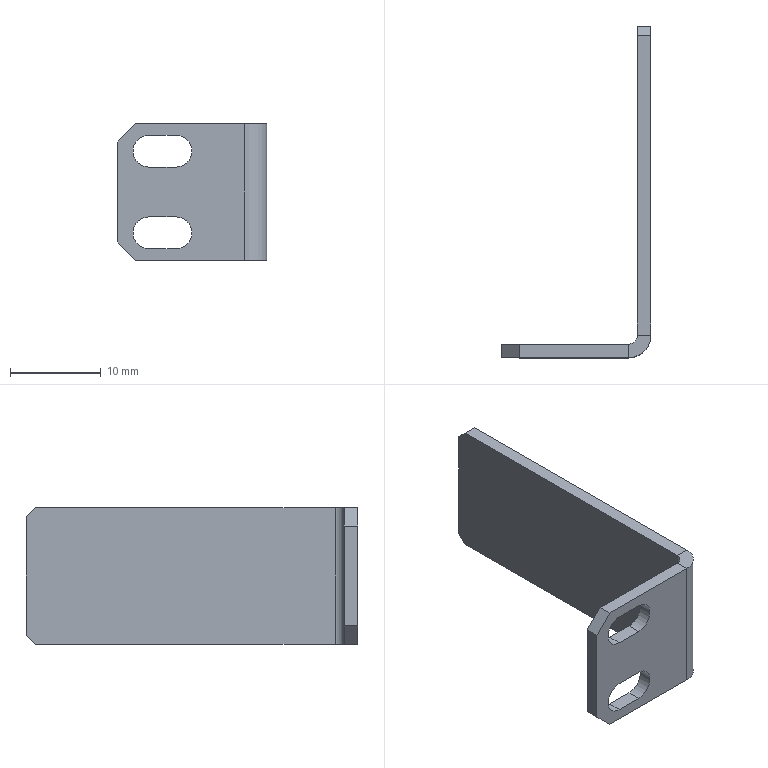Part | NX | 1 solid | 26 faces | box 16.5 x 36.5 x 15 mm | volume 1074 mm3 | plane 20 | cylinder 6 | commonest cylinder face diameters 3.5 x4 2 x1 5 x1
STEP:
#1=CARTESIAN_POINT('',(6.5,-1.5,-7.5));
#2=VERTEX_POINT('',#1);
#3=CARTESIAN_POINT('',(-5.5,-1.5,-7.5));
#4=VERTEX_POINT('',#3);
#5=CARTESIAN_POINT('',(-7.5,-1.5,-7.5));
#6=DIRECTION('',(-1.,0.,0.));
#7=VECTOR('',#6,1000.);
#8=LINE('',#5,#7);
#9=EDGE_CURVE('',#2,#4,#8,.T.);
#10=ORIENTED_EDGE('',*,*,#9,.T.);
#11=CARTESIAN_POINT('',(-5.5,0.,-7.5));
#12=VERTEX_POINT('',#11);
#13=CARTESIAN_POINT('',(-5.5,-1.5,-7.5));
#14=DIRECTION('',(0.,1.,0.));
#15=VECTOR('',#14,1000.);
#16=LINE('',#13,#15);
#17=EDGE_CURVE('',#4,#12,#16,.T.);
#18=ORIENTED_EDGE('',*,*,#17,.T.);
#19=CARTESIAN_POINT('',(6.5,0.,-7.5));
#20=VERTEX_POINT('',#19);
#21=CARTESIAN_POINT('',(-7.5,0.,-7.5));
#22=DIRECTION('',(-1.,0.,0.));
#23=VECTOR('',#22,1000.);
#24=LINE('',#21,#23);
#25=EDGE_CURVE('',#20,#12,#24,.T.);
#26=ORIENTED_EDGE('',*,*,#25,.F.);
#27=CARTESIAN_POINT('',(6.5,0.,-7.5));
#28=DIRECTION('',(0.,-1.,0.));
#29=VECTOR('',#28,1000.);
#30=LINE('',#27,#29);
#31=EDGE_CURVE('',#20,#2,#30,.T.);
#32=ORIENTED_EDGE('',*,*,#31,.T.);
#33=EDGE_LOOP('',(#10,#18,#26,#32));
#34=FACE_BOUND('',#33,.T.);
#35=CARTESIAN_POINT('',(-7.5,-1.5,-7.5));
#36=DIRECTION('',(0.,0.,-1.));
#37=DIRECTION('',(-1.,0.,0.));
#38=AXIS2_PLACEMENT_3D('',#35,#36,#37);
#39=PLANE('',#38);
#40=ADVANCED_FACE('',(#34),#39,.T.);
#41=CARTESIAN_POINT('',(-4.,-1.5,6.25));
#42=VERTEX_POINT('',#41);
#43=CARTESIAN_POINT('',(-4.,-1.5,2.75));
#44=VERTEX_POINT('',#43);
#45=CARTESIAN_POINT('',(-4.,-1.5,4.5));
#46=DIRECTION('',(0.,-1.,0.));
#47=DIRECTION('',(0.,0.,-1.));
#48=AXIS2_PLACEMENT_3D('',#45,#46,#47);
#49=CIRCLE('',#48,1.75);
#50=EDGE_CURVE('',#42,#44,#49,.T.);
#51=ORIENTED_EDGE('',*,*,#50,.F.);
#52=CARTESIAN_POINT('',(-1.,-1.5,6.25));
#53=VERTEX_POINT('',#52);
#54=CARTESIAN_POINT('',(-4.,-1.5,6.25));
#55=DIRECTION('',(-1.,0.,0.));
#56=VECTOR('',#55,1000.);
#57=LINE('',#54,#56);
#58=EDGE_CURVE('',#53,#42,#57,.T.);
#59=ORIENTED_EDGE('',*,*,#58,.F.);
#60=CARTESIAN_POINT('',(-1.,-1.5,2.75));
#61=VERTEX_POINT('',#60);
#62=CARTESIAN_POINT('',(-1.,-1.5,4.5));
#63=DIRECTION('',(0.,-1.,0.));
#64=DIRECTION('',(0.,0.,-1.));
#65=AXIS2_PLACEMENT_3D('',#62,#63,#64);
#66=CIRCLE('',#65,1.75);
#67=EDGE_CURVE('',#61,#53,#66,.T.);
#68=ORIENTED_EDGE('',*,*,#67,.F.);
#69=CARTESIAN_POINT('',(-4.,-1.5,2.75));
#70=DIRECTION('',(1.,0.,0.));
#71=VECTOR('',#70,1000.);
#72=LINE('',#69,#71);
#73=EDGE_CURVE('',#44,#61,#72,.T.);
#74=ORIENTED_EDGE('',*,*,#73,.F.);
#75=EDGE_LOOP('',(#51,#59,#68,#74));
#76=FACE_BOUND('',#75,.T.);
#77=CARTESIAN_POINT('',(-4.,-1.5,-2.75));
#78=VERTEX_POINT('',#77);
#79=CARTESIAN_POINT('',(-4.,-1.5,-6.25));
#80=VERTEX_POINT('',#79);
#81=CARTESIAN_POINT('',(-4.,-1.5,-4.5));
#82=DIRECTION('',(0.,-1.,0.));
#83=DIRECTION('',(0.,0.,-1.));
#84=AXIS2_PLACEMENT_3D('',#81,#82,#83);
#85=CIRCLE('',#84,1.75);
#86=EDGE_CURVE('',#78,#80,#85,.T.);
#87=ORIENTED_EDGE('',*,*,#86,.F.);
#88=CARTESIAN_POINT('',(-1.,-1.5,-2.75));
#89=VERTEX_POINT('',#88);
#90=CARTESIAN_POINT('',(-4.,-1.5,-2.75));
#91=DIRECTION('',(-1.,0.,0.));
#92=VECTOR('',#91,1000.);
#93=LINE('',#90,#92);
#94=EDGE_CURVE('',#89,#78,#93,.T.);
#95=ORIENTED_EDGE('',*,*,#94,.F.);
#96=CARTESIAN_POINT('',(-1.,-1.5,-6.25));
#97=VERTEX_POINT('',#96);
#98=CARTESIAN_POINT('',(-1.,-1.5,-4.5));
#99=DIRECTION('',(0.,-1.,0.));
#100=DIRECTION('',(0.,0.,-1.));
#101=AXIS2_PLACEMENT_3D('',#98,#99,#100);
#102=CIRCLE('',#101,1.75);
#103=EDGE_CURVE('',#97,#89,#102,.T.);
#104=ORIENTED_EDGE('',*,*,#103,.F.);
#105=CARTESIAN_POINT('',(-4.,-1.5,-6.25));
#106=DIRECTION('',(1.,0.,0.));
#107=VECTOR('',#106,1000.);
#108=LINE('',#105,#107);
#109=EDGE_CURVE('',#80,#97,#108,.T.);
#110=ORIENTED_EDGE('',*,*,#109,.F.);
#111=EDGE_LOOP('',(#87,#95,#104,#110));
#112=FACE_BOUND('',#111,.T.);
#113=CARTESIAN_POINT('',(-5.5,-1.5,7.5));
#114=VERTEX_POINT('',#113);
#115=CARTESIAN_POINT('',(6.5,-1.5,7.5));
#116=VERTEX_POINT('',#115);
#117=CARTESIAN_POINT('',(-7.5,-1.5,7.5));
#118=DIRECTION('',(1.,0.,0.));
#119=VECTOR('',#118,1000.);
#120=LINE('',#117,#119);
#121=EDGE_CURVE('',#114,#116,#120,.T.);
#122=ORIENTED_EDGE('',*,*,#121,.F.);
#123=CARTESIAN_POINT('',(-7.5,-1.5,5.5));
#124=VERTEX_POINT('',#123);
#125=CARTESIAN_POINT('',(-6.5,-1.5,6.5));
#126=DIRECTION('',(0.7071,0.,0.7071));
#127=VECTOR('',#126,1000.);
#128=LINE('',#125,#127);
#129=EDGE_CURVE('',#114,#124,#128,.F.);
#130=ORIENTED_EDGE('',*,*,#129,.T.);
#131=CARTESIAN_POINT('',(-7.5,-1.5,-5.5));
#132=VERTEX_POINT('',#131);
#133=CARTESIAN_POINT('',(-7.5,-1.5,7.5));
#134=DIRECTION('',(0.,0.,1.));
#135=VECTOR('',#134,1000.);
#136=LINE('',#133,#135);
#137=EDGE_CURVE('',#132,#124,#136,.T.);
#138=ORIENTED_EDGE('',*,*,#137,.F.);
#139=CARTESIAN_POINT('',(-6.5,-1.5,-6.5));
#140=DIRECTION('',(-0.7071,0.,0.7071));
#141=VECTOR('',#140,1000.);
#142=LINE('',#139,#141);
#143=EDGE_CURVE('',#132,#4,#142,.F.);
#144=ORIENTED_EDGE('',*,*,#143,.T.);
#145=ORIENTED_EDGE('',*,*,#9,.F.);
#146=CARTESIAN_POINT('',(6.5,-1.5,-7.5));
#147=DIRECTION('',(0.,0.,-1.));
#148=VECTOR('',#147,1000.);
#149=LINE('',#146,#148);
#150=EDGE_CURVE('',#2,#116,#149,.F.);
#151=ORIENTED_EDGE('',*,*,#150,.T.);
#152=EDGE_LOOP('',(#122,#130,#138,#144,#145,#151));
#153=FACE_BOUND('',#152,.T.);
#154=CARTESIAN_POINT('',(0.,-1.5,0.));
#155=DIRECTION('',(0.,-1.,0.));
#156=DIRECTION('',(0.,0.,-1.));
#157=AXIS2_PLACEMENT_3D('',#154,#155,#156);
#158=PLANE('',#157);
#159=ADVANCED_FACE('',(#76,#112,#153),#158,.T.);
#160=CARTESIAN_POINT('',(-1.,0.,6.25));
#161=VERTEX_POINT('',#160);
#162=CARTESIAN_POINT('',(-4.,0.,6.25));
#163=VERTEX_POINT('',#162);
#164=CARTESIAN_POINT('',(0.,0.,6.25));
#165=DIRECTION('',(-1.,0.,0.));
#166=VECTOR('',#165,1000.);
#167=LINE('',#164,#166);
#168=EDGE_CURVE('',#161,#163,#167,.T.);
#169=ORIENTED_EDGE('',*,*,#168,.T.);
#170=CARTESIAN_POINT('',(-4.,0.,2.75));
#171=VERTEX_POINT('',#170);
#172=CARTESIAN_POINT('',(-4.,0.,4.5));
#173=DIRECTION('',(0.,-1.,0.));
#174=DIRECTION('',(0.,0.,-1.));
#175=AXIS2_PLACEMENT_3D('',#172,#173,#174);
#176=CIRCLE('',#175,1.75);
#177=EDGE_CURVE('',#163,#171,#176,.T.);
#178=ORIENTED_EDGE('',*,*,#177,.T.);
#179=CARTESIAN_POINT('',(-1.,0.,2.75));
#180=VERTEX_POINT('',#179);
#181=CARTESIAN_POINT('',(0.,0.,2.75));
#182=DIRECTION('',(1.,0.,0.));
#183=VECTOR('',#182,1000.);
#184=LINE('',#181,#183);
#185=EDGE_CURVE('',#171,#180,#184,.T.);
#186=ORIENTED_EDGE('',*,*,#185,.T.);
#187=CARTESIAN_POINT('',(-1.,0.,4.5));
#188=DIRECTION('',(0.,-1.,0.));
#189=DIRECTION('',(0.,0.,-1.));
#190=AXIS2_PLACEMENT_3D('',#187,#188,#189);
#191=CIRCLE('',#190,1.75);
#192=EDGE_CURVE('',#180,#161,#191,.T.);
#193=ORIENTED_EDGE('',*,*,#192,.T.);
#194=EDGE_LOOP('',(#169,#178,#186,#193));
#195=FACE_BOUND('',#194,.T.);
#196=CARTESIAN_POINT('',(-1.,0.,-2.75));
#197=VERTEX_POINT('',#196);
#198=CARTESIAN_POINT('',(-4.,0.,-2.75));
#199=VERTEX_POINT('',#198);
#200=CARTESIAN_POINT('',(0.,0.,-2.75));
#201=DIRECTION('',(-1.,0.,0.));
#202=VECTOR('',#201,1000.);
#203=LINE('',#200,#202);
#204=EDGE_CURVE('',#197,#199,#203,.T.);
#205=ORIENTED_EDGE('',*,*,#204,.T.);
#206=CARTESIAN_POINT('',(-4.,0.,-6.25));
#207=VERTEX_POINT('',#206);
#208=CARTESIAN_POINT('',(-4.,0.,-4.5));
#209=DIRECTION('',(0.,-1.,0.));
#210=DIRECTION('',(0.,0.,-1.));
#211=AXIS2_PLACEMENT_3D('',#208,#209,#210);
#212=CIRCLE('',#211,1.75);
#213=EDGE_CURVE('',#199,#207,#212,.T.);
#214=ORIENTED_EDGE('',*,*,#213,.T.);
#215=CARTESIAN_POINT('',(-1.,0.,-6.25));
#216=VERTEX_POINT('',#215);
#217=CARTESIAN_POINT('',(0.,0.,-6.25));
#218=DIRECTION('',(1.,0.,0.));
#219=VECTOR('',#218,1000.);
#220=LINE('',#217,#219);
#221=EDGE_CURVE('',#207,#216,#220,.T.);
#222=ORIENTED_EDGE('',*,*,#221,.T.);
#223=CARTESIAN_POINT('',(-1.,0.,-4.5));
#224=DIRECTION('',(0.,-1.,0.));
#225=DIRECTION('',(0.,0.,-1.));
#226=AXIS2_PLACEMENT_3D('',#223,#224,#225);
#227=CIRCLE('',#226,1.75);
#228=EDGE_CURVE('',#216,#197,#227,.T.);
#229=ORIENTED_EDGE('',*,*,#228,.T.);
#230=EDGE_LOOP('',(#205,#214,#222,#229));
#231=FACE_BOUND('',#230,.T.);
#232=CARTESIAN_POINT('',(-7.5,0.,-5.5));
#233=VERTEX_POINT('',#232);
#234=CARTESIAN_POINT('',(-7.5,0.,5.5));
#235=VERTEX_POINT('',#234);
#236=CARTESIAN_POINT('',(-7.5,0.,7.5));
#237=DIRECTION('',(0.,0.,1.));
#238=VECTOR('',#237,1000.);
#239=LINE('',#236,#238);
#240=EDGE_CURVE('',#233,#235,#239,.T.);
#241=ORIENTED_EDGE('',*,*,#240,.T.);
#242=CARTESIAN_POINT('',(-5.5,0.,7.5));
#243=VERTEX_POINT('',#242);
#244=CARTESIAN_POINT('',(-7.5,0.,5.5));
#245=DIRECTION('',(-0.7071,0.,-0.7071));
#246=VECTOR('',#245,1000.);
#247=LINE('',#244,#246);
#248=EDGE_CURVE('',#235,#243,#247,.F.);
#249=ORIENTED_EDGE('',*,*,#248,.T.);
#250=CARTESIAN_POINT('',(6.5,0.,7.5));
#251=VERTEX_POINT('',#250);
#252=CARTESIAN_POINT('',(-7.5,0.,7.5));
#253=DIRECTION('',(1.,0.,0.));
#254=VECTOR('',#253,1000.);
#255=LINE('',#252,#254);
#256=EDGE_CURVE('',#243,#251,#255,.T.);
#257=ORIENTED_EDGE('',*,*,#256,.T.);
#258=CARTESIAN_POINT('',(6.5,0.,-7.5));
#259=DIRECTION('',(0.,0.,-1.));
#260=VECTOR('',#259,1000.);
#261=LINE('',#258,#260);
#262=EDGE_CURVE('',#20,#251,#261,.F.);
#263=ORIENTED_EDGE('',*,*,#262,.F.);
#264=ORIENTED_EDGE('',*,*,#25,.T.);
#265=CARTESIAN_POINT('',(-5.5,0.,-7.5));
#266=DIRECTION('',(0.7071,0.,-0.7071));
#267=VECTOR('',#266,1000.);
#268=LINE('',#265,#267);
#269=EDGE_CURVE('',#12,#233,#268,.F.);
#270=ORIENTED_EDGE('',*,*,#269,.T.);
#271=EDGE_LOOP('',(#241,#249,#257,#263,#264,#270));
#272=FACE_BOUND('',#271,.T.);
#273=CARTESIAN_POINT('',(0.,0.,0.));
#274=DIRECTION('',(0.,-1.,0.));
#275=DIRECTION('',(0.,0.,-1.));
#276=AXIS2_PLACEMENT_3D('',#273,#274,#275);
#277=PLANE('',#276);
#278=ADVANCED_FACE('',(#195,#231,#272),#277,.F.);
#279=ORIENTED_EDGE('',*,*,#256,.F.);
#280=CARTESIAN_POINT('',(-5.5,-1.5,7.5));
#281=DIRECTION('',(0.,-1.,0.));
#282=VECTOR('',#281,1000.);
#283=LINE('',#280,#282);
#284=EDGE_CURVE('',#243,#114,#283,.T.);
#285=ORIENTED_EDGE('',*,*,#284,.T.);
#286=ORIENTED_EDGE('',*,*,#121,.T.);
#287=CARTESIAN_POINT('',(6.5,0.,7.5));
#288=DIRECTION('',(0.,-1.,0.));
#289=VECTOR('',#288,1000.);
#290=LINE('',#287,#289);
#291=EDGE_CURVE('',#251,#116,#290,.T.);
#292=ORIENTED_EDGE('',*,*,#291,.F.);
#293=EDGE_LOOP('',(#279,#285,#286,#292));
#294=FACE_BOUND('',#293,.T.);
#295=CARTESIAN_POINT('',(-7.5,-1.5,7.5));
#296=DIRECTION('',(0.,0.,1.));
#297=DIRECTION('',(1.,0.,0.));
#298=AXIS2_PLACEMENT_3D('',#295,#296,#297);
#299=PLANE('',#298);
#300=ADVANCED_FACE('',(#294),#299,.T.);
#301=ORIENTED_EDGE('',*,*,#137,.T.);
#302=CARTESIAN_POINT('',(-7.5,-1.5,5.5));
#303=DIRECTION('',(0.,1.,0.));
#304=VECTOR('',#303,1000.);
#305=LINE('',#302,#304);
#306=EDGE_CURVE('',#124,#235,#305,.T.);
#307=ORIENTED_EDGE('',*,*,#306,.T.);
#308=ORIENTED_EDGE('',*,*,#240,.F.);
#309=CARTESIAN_POINT('',(-7.5,-1.5,-5.5));
#310=DIRECTION('',(0.,-1.,0.));
#311=VECTOR('',#310,1000.);
#312=LINE('',#309,#311);
#313=EDGE_CURVE('',#233,#132,#312,.T.);
#314=ORIENTED_EDGE('',*,*,#313,.T.);
#315=EDGE_LOOP('',(#301,#307,#308,#314));
#316=FACE_BOUND('',#315,.T.);
#317=CARTESIAN_POINT('',(-7.5,-1.5,7.5));
#318=DIRECTION('',(-1.,0.,0.));
#319=DIRECTION('',(0.,0.,1.));
#320=AXIS2_PLACEMENT_3D('',#317,#318,#319);
#321=PLANE('',#320);
#322=ADVANCED_FACE('',(#316),#321,.T.);
#323=CARTESIAN_POINT('',(7.5,1.,7.5));
#324=VERTEX_POINT('',#323);
#325=CARTESIAN_POINT('',(9.,1.,7.5));
#326=VERTEX_POINT('',#325);
#327=CARTESIAN_POINT('',(7.5,1.,7.5));
#328=DIRECTION('',(1.,0.,0.));
#329=VECTOR('',#328,1000.);
#330=LINE('',#327,#329);
#331=EDGE_CURVE('',#324,#326,#330,.T.);
#332=ORIENTED_EDGE('',*,*,#331,.F.);
#333=CARTESIAN_POINT('',(6.5,1.,7.5));
#334=DIRECTION('',(0.,0.,-1.));
#335=DIRECTION('',(-1.,0.,0.));
#336=AXIS2_PLACEMENT_3D('',#333,#334,#335);
#337=CIRCLE('',#336,1.);
#338=EDGE_CURVE('',#251,#324,#337,.F.);
#339=ORIENTED_EDGE('',*,*,#338,.F.);
#340=ORIENTED_EDGE('',*,*,#291,.T.);
#341=CARTESIAN_POINT('',(6.5,1.,7.5));
#342=DIRECTION('',(0.,0.,-1.));
#343=DIRECTION('',(-1.,0.,0.));
#344=AXIS2_PLACEMENT_3D('',#341,#342,#343);
#345=CIRCLE('',#344,2.5);
#346=EDGE_CURVE('',#116,#326,#345,.F.);
#347=ORIENTED_EDGE('',*,*,#346,.T.);
#348=EDGE_LOOP('',(#332,#339,#340,#347));
#349=FACE_BOUND('',#348,.T.);
#350=CARTESIAN_POINT('',(6.5,1.,7.5));
#351=DIRECTION('',(0.,0.,1.));
#352=DIRECTION('',(1.,0.,0.));
#353=AXIS2_PLACEMENT_3D('',#350,#351,#352);
#354=PLANE('',#353);
#355=ADVANCED_FACE('',(#349),#354,.T.);
#356=CARTESIAN_POINT('',(7.5,1.,-7.5));
#357=VERTEX_POINT('',#356);
#358=CARTESIAN_POINT('',(6.5,1.,-7.5));
#359=DIRECTION('',(0.,0.,-1.));
#360=DIRECTION('',(-1.,0.,0.));
#361=AXIS2_PLACEMENT_3D('',#358,#359,#360);
#362=CIRCLE('',#361,1.);
#363=EDGE_CURVE('',#357,#20,#362,.T.);
#364=ORIENTED_EDGE('',*,*,#363,.F.);
#365=CARTESIAN_POINT('',(9.,1.,-7.5));
#366=VERTEX_POINT('',#365);
#367=CARTESIAN_POINT('',(7.5,1.,-7.5));
#368=DIRECTION('',(1.,0.,0.));
#369=VECTOR('',#368,1000.);
#370=LINE('',#367,#369);
#371=EDGE_CURVE('',#357,#366,#370,.T.);
#372=ORIENTED_EDGE('',*,*,#371,.T.);
#373=CARTESIAN_POINT('',(6.5,1.,-7.5));
#374=DIRECTION('',(0.,0.,-1.));
#375=DIRECTION('',(-1.,0.,0.));
#376=AXIS2_PLACEMENT_3D('',#373,#374,#375);
#377=CIRCLE('',#376,2.5);
#378=EDGE_CURVE('',#366,#2,#377,.T.);
#379=ORIENTED_EDGE('',*,*,#378,.T.);
#380=ORIENTED_EDGE('',*,*,#31,.F.);
#381=EDGE_LOOP('',(#364,#372,#379,#380));
#382=FACE_BOUND('',#381,.T.);
#383=CARTESIAN_POINT('',(6.5,1.,-7.5));
#384=DIRECTION('',(0.,0.,1.));
#385=DIRECTION('',(1.,0.,0.));
#386=AXIS2_PLACEMENT_3D('',#383,#384,#385);
#387=PLANE('',#386);
#388=ADVANCED_FACE('',(#382),#387,.F.);
#389=ORIENTED_EDGE('',*,*,#150,.F.);
#390=ORIENTED_EDGE('',*,*,#378,.F.);
#391=CARTESIAN_POINT('',(9.,1.,0.));
#392=DIRECTION('',(0.,0.,1.));
#393=VECTOR('',#392,1000.);
#394=LINE('',#391,#393);
#395=EDGE_CURVE('',#366,#326,#394,.T.);
#396=ORIENTED_EDGE('',*,*,#395,.T.);
#397=ORIENTED_EDGE('',*,*,#346,.F.);
#398=EDGE_LOOP('',(#389,#390,#396,#397));
#399=FACE_BOUND('',#398,.T.);
#400=CARTESIAN_POINT('',(6.5,1.,-7.5));
#401=DIRECTION('',(0.,0.,-1.));
#402=DIRECTION('',(1.,0.,0.));
#403=AXIS2_PLACEMENT_3D('',#400,#401,#402);
#404=CYLINDRICAL_SURFACE('',#403,2.5);
#405=ADVANCED_FACE('',(#399),#404,.T.);
#406=ORIENTED_EDGE('',*,*,#262,.T.);
#407=ORIENTED_EDGE('',*,*,#338,.T.);
#408=CARTESIAN_POINT('',(7.5,1.,7.5));
#409=DIRECTION('',(0.,0.,-1.));
#410=VECTOR('',#409,1000.);
#411=LINE('',#408,#410);
#412=EDGE_CURVE('',#324,#357,#411,.T.);
#413=ORIENTED_EDGE('',*,*,#412,.T.);
#414=ORIENTED_EDGE('',*,*,#363,.T.);
#415=EDGE_LOOP('',(#406,#407,#413,#414));
#416=FACE_BOUND('',#415,.T.);
#417=CARTESIAN_POINT('',(6.5,1.,-7.5));
#418=DIRECTION('',(0.,0.,-1.));
#419=DIRECTION('',(1.,0.,0.));
#420=AXIS2_PLACEMENT_3D('',#417,#418,#419);
#421=CYLINDRICAL_SURFACE('',#420,1.);
#422=ADVANCED_FACE('',(#416),#421,.F.);
#423=CARTESIAN_POINT('',(9.,34.,7.5));
#424=VERTEX_POINT('',#423);
#425=CARTESIAN_POINT('',(9.,0.,7.5));
#426=DIRECTION('',(0.,-1.,0.));
#427=VECTOR('',#426,1000.);
#428=LINE('',#425,#427);
#429=EDGE_CURVE('',#424,#326,#428,.T.);
#430=ORIENTED_EDGE('',*,*,#429,.F.);
#431=CARTESIAN_POINT('',(7.5,34.,7.5));
#432=VERTEX_POINT('',#431);
#433=CARTESIAN_POINT('',(9.,34.,7.5));
#434=DIRECTION('',(-1.,0.,0.));
#435=VECTOR('',#434,1000.);
#436=LINE('',#433,#435);
#437=EDGE_CURVE('',#424,#432,#436,.T.);
#438=ORIENTED_EDGE('',*,*,#437,.T.);
#439=CARTESIAN_POINT('',(7.5,0.,7.5));
#440=DIRECTION('',(0.,-1.,0.));
#441=VECTOR('',#440,1000.);
#442=LINE('',#439,#441);
#443=EDGE_CURVE('',#432,#324,#442,.T.);
#444=ORIENTED_EDGE('',*,*,#443,.T.);
#445=ORIENTED_EDGE('',*,*,#331,.T.);
#446=EDGE_LOOP('',(#430,#438,#444,#445));
#447=FACE_BOUND('',#446,.T.);
#448=CARTESIAN_POINT('',(9.,0.,7.5));
#449=DIRECTION('',(0.,0.,-1.));
#450=DIRECTION('',(0.,1.,0.));
#451=AXIS2_PLACEMENT_3D('',#448,#449,#450);
#452=PLANE('',#451);
#453=ADVANCED_FACE('',(#447),#452,.F.);
#454=CARTESIAN_POINT('',(7.5,34.,-7.5));
#455=VERTEX_POINT('',#454);
#456=CARTESIAN_POINT('',(7.5,35.,-7.5));
#457=DIRECTION('',(0.,1.,0.));
#458=VECTOR('',#457,1000.);
#459=LINE('',#456,#458);
#460=EDGE_CURVE('',#357,#455,#459,.T.);
#461=ORIENTED_EDGE('',*,*,#460,.T.);
#462=CARTESIAN_POINT('',(9.,34.,-7.5));
#463=VERTEX_POINT('',#462);
#464=CARTESIAN_POINT('',(9.,34.,-7.5));
#465=DIRECTION('',(1.,0.,0.));
#466=VECTOR('',#465,1000.);
#467=LINE('',#464,#466);
#468=EDGE_CURVE('',#455,#463,#467,.T.);
#469=ORIENTED_EDGE('',*,*,#468,.T.);
#470=CARTESIAN_POINT('',(9.,35.,-7.5));
#471=DIRECTION('',(0.,1.,0.));
#472=VECTOR('',#471,1000.);
#473=LINE('',#470,#472);
#474=EDGE_CURVE('',#366,#463,#473,.T.);
#475=ORIENTED_EDGE('',*,*,#474,.F.);
#476=ORIENTED_EDGE('',*,*,#371,.F.);
#477=EDGE_LOOP('',(#461,#469,#475,#476));
#478=FACE_BOUND('',#477,.T.);
#479=CARTESIAN_POINT('',(9.,35.,-7.5));
#480=DIRECTION('',(0.,0.,1.));
#481=DIRECTION('',(0.,-1.,0.));
#482=AXIS2_PLACEMENT_3D('',#479,#480,#481);
#483=PLANE('',#482);
#484=ADVANCED_FACE('',(#478),#483,.F.);
#485=CARTESIAN_POINT('',(9.,35.,-6.5));
#486=VERTEX_POINT('',#485);
#487=CARTESIAN_POINT('',(9.,35.,6.5));
#488=VERTEX_POINT('',#487);
#489=CARTESIAN_POINT('',(9.,35.,7.5));
#490=DIRECTION('',(0.,0.,1.));
#491=VECTOR('',#490,1000.);
#492=LINE('',#489,#491);
#493=EDGE_CURVE('',#486,#488,#492,.T.);
#494=ORIENTED_EDGE('',*,*,#493,.T.);
#495=CARTESIAN_POINT('',(9.,34.,7.5));
#496=DIRECTION('',(0.,0.7071,-0.7071));
#497=VECTOR('',#496,1000.);
#498=LINE('',#495,#497);
#499=EDGE_CURVE('',#488,#424,#498,.F.);
#500=ORIENTED_EDGE('',*,*,#499,.T.);
#501=ORIENTED_EDGE('',*,*,#429,.T.);
#502=ORIENTED_EDGE('',*,*,#395,.F.);
#503=ORIENTED_EDGE('',*,*,#474,.T.);
#504=CARTESIAN_POINT('',(9.,35.,-6.5));
#505=DIRECTION('',(0.,-0.7071,-0.7071));
#506=VECTOR('',#505,1000.);
#507=LINE('',#504,#506);
#508=EDGE_CURVE('',#463,#486,#507,.F.);
#509=ORIENTED_EDGE('',*,*,#508,.T.);
#510=EDGE_LOOP('',(#494,#500,#501,#502,#503,#509));
#511=FACE_BOUND('',#510,.T.);
#512=CARTESIAN_POINT('',(9.,0.,0.));
#513=DIRECTION('',(-1.,0.,0.));
#514=DIRECTION('',(0.,-1.,0.));
#515=AXIS2_PLACEMENT_3D('',#512,#513,#514);
#516=PLANE('',#515);
#517=ADVANCED_FACE('',(#511),#516,.F.);
#518=ORIENTED_EDGE('',*,*,#443,.F.);
#519=CARTESIAN_POINT('',(7.5,35.,6.5));
#520=VERTEX_POINT('',#519);
#521=CARTESIAN_POINT('',(7.5,20.75,20.75));
#522=DIRECTION('',(0.,-0.7071,0.7071));
#523=VECTOR('',#522,1000.);
#524=LINE('',#521,#523);
#525=EDGE_CURVE('',#432,#520,#524,.F.);
#526=ORIENTED_EDGE('',*,*,#525,.T.);
#527=CARTESIAN_POINT('',(7.5,35.,-6.5));
#528=VERTEX_POINT('',#527);
#529=CARTESIAN_POINT('',(7.5,35.,7.5));
#530=DIRECTION('',(0.,0.,1.));
#531=VECTOR('',#530,1000.);
#532=LINE('',#529,#531);
#533=EDGE_CURVE('',#528,#520,#532,.T.);
#534=ORIENTED_EDGE('',*,*,#533,.F.);
#535=CARTESIAN_POINT('',(7.5,20.75,-20.75));
#536=DIRECTION('',(0.,0.7071,0.7071));
#537=VECTOR('',#536,1000.);
#538=LINE('',#535,#537);
#539=EDGE_CURVE('',#528,#455,#538,.F.);
#540=ORIENTED_EDGE('',*,*,#539,.T.);
#541=ORIENTED_EDGE('',*,*,#460,.F.);
#542=ORIENTED_EDGE('',*,*,#412,.F.);
#543=EDGE_LOOP('',(#518,#526,#534,#540,#541,#542));
#544=FACE_BOUND('',#543,.T.);
#545=CARTESIAN_POINT('',(7.5,0.,0.));
#546=DIRECTION('',(-1.,0.,0.));
#547=DIRECTION('',(0.,-1.,0.));
#548=AXIS2_PLACEMENT_3D('',#545,#546,#547);
#549=PLANE('',#548);
#550=ADVANCED_FACE('',(#544),#549,.T.);
#551=ORIENTED_EDGE('',*,*,#533,.T.);
#552=CARTESIAN_POINT('',(9.,35.,6.5));
#553=DIRECTION('',(1.,0.,0.));
#554=VECTOR('',#553,1000.);
#555=LINE('',#552,#554);
#556=EDGE_CURVE('',#520,#488,#555,.T.);
#557=ORIENTED_EDGE('',*,*,#556,.T.);
#558=ORIENTED_EDGE('',*,*,#493,.F.);
#559=CARTESIAN_POINT('',(9.,35.,-6.5));
#560=DIRECTION('',(-1.,0.,0.));
#561=VECTOR('',#560,1000.);
#562=LINE('',#559,#561);
#563=EDGE_CURVE('',#486,#528,#562,.T.);
#564=ORIENTED_EDGE('',*,*,#563,.T.);
#565=EDGE_LOOP('',(#551,#557,#558,#564));
#566=FACE_BOUND('',#565,.T.);
#567=CARTESIAN_POINT('',(9.,35.,7.5));
#568=DIRECTION('',(0.,-1.,0.));
#569=DIRECTION('',(1.,0.,0.));
#570=AXIS2_PLACEMENT_3D('',#567,#568,#569);
#571=PLANE('',#570);
#572=ADVANCED_FACE('',(#566),#571,.F.);
#573=ORIENTED_EDGE('',*,*,#129,.F.);
#574=ORIENTED_EDGE('',*,*,#284,.F.);
#575=ORIENTED_EDGE('',*,*,#248,.F.);
#576=ORIENTED_EDGE('',*,*,#306,.F.);
#577=EDGE_LOOP('',(#573,#574,#575,#576));
#578=FACE_BOUND('',#577,.T.);
#579=CARTESIAN_POINT('',(-7.5,-1.5,5.5));
#580=DIRECTION('',(0.7071,0.,-0.7071));
#581=DIRECTION('',(0.,1.,0.));
#582=AXIS2_PLACEMENT_3D('',#579,#580,#581);
#583=PLANE('',#582);
#584=ADVANCED_FACE('',(#578),#583,.F.);
#585=ORIENTED_EDGE('',*,*,#143,.F.);
#586=ORIENTED_EDGE('',*,*,#313,.F.);
#587=ORIENTED_EDGE('',*,*,#269,.F.);
#588=ORIENTED_EDGE('',*,*,#17,.F.);
#589=EDGE_LOOP('',(#585,#586,#587,#588));
#590=FACE_BOUND('',#589,.T.);
#591=CARTESIAN_POINT('',(-5.5,-1.5,-7.5));
#592=DIRECTION('',(0.7071,0.,0.7071));
#593=DIRECTION('',(0.,1.,0.));
#594=AXIS2_PLACEMENT_3D('',#591,#592,#593);
#595=PLANE('',#594);
#596=ADVANCED_FACE('',(#590),#595,.F.);
#597=CARTESIAN_POINT('',(-4.,35.,-2.75));
#598=DIRECTION('',(0.,-1.,0.));
#599=VECTOR('',#598,1000.);
#600=LINE('',#597,#599);
#601=EDGE_CURVE('',#199,#78,#600,.T.);
#602=ORIENTED_EDGE('',*,*,#601,.T.);
#603=ORIENTED_EDGE('',*,*,#86,.T.);
#604=CARTESIAN_POINT('',(-4.,35.,-6.25));
#605=DIRECTION('',(0.,-1.,0.));
#606=VECTOR('',#605,1000.);
#607=LINE('',#604,#606);
#608=EDGE_CURVE('',#207,#80,#607,.T.);
#609=ORIENTED_EDGE('',*,*,#608,.F.);
#610=ORIENTED_EDGE('',*,*,#213,.F.);
#611=EDGE_LOOP('',(#602,#603,#609,#610));
#612=FACE_BOUND('',#611,.T.);
#613=CARTESIAN_POINT('',(-4.,35.,-4.5));
#614=DIRECTION('',(0.,-1.,0.));
#615=DIRECTION('',(0.,0.,-1.));
#616=AXIS2_PLACEMENT_3D('',#613,#614,#615);
#617=CYLINDRICAL_SURFACE('',#616,1.75);
#618=ADVANCED_FACE('',(#612),#617,.F.);
#619=CARTESIAN_POINT('',(-1.,35.,-2.75));
#620=DIRECTION('',(0.,-1.,0.));
#621=VECTOR('',#620,1000.);
#622=LINE('',#619,#621);
#623=EDGE_CURVE('',#197,#89,#622,.T.);
#624=ORIENTED_EDGE('',*,*,#623,.T.);
#625=ORIENTED_EDGE('',*,*,#94,.T.);
#626=ORIENTED_EDGE('',*,*,#601,.F.);
#627=ORIENTED_EDGE('',*,*,#204,.F.);
#628=EDGE_LOOP('',(#624,#625,#626,#627));
#629=FACE_BOUND('',#628,.T.);
#630=CARTESIAN_POINT('',(-4.,35.,-2.75));
#631=DIRECTION('',(0.,0.,1.));
#632=DIRECTION('',(1.,0.,0.));
#633=AXIS2_PLACEMENT_3D('',#630,#631,#632);
#634=PLANE('',#633);
#635=ADVANCED_FACE('',(#629),#634,.F.);
#636=CARTESIAN_POINT('',(-1.,35.,-6.25));
#637=DIRECTION('',(0.,-1.,0.));
#638=VECTOR('',#637,1000.);
#639=LINE('',#636,#638);
#640=EDGE_CURVE('',#216,#97,#639,.T.);
#641=ORIENTED_EDGE('',*,*,#640,.T.);
#642=ORIENTED_EDGE('',*,*,#103,.T.);
#643=ORIENTED_EDGE('',*,*,#623,.F.);
#644=ORIENTED_EDGE('',*,*,#228,.F.);
#645=EDGE_LOOP('',(#641,#642,#643,#644));
#646=FACE_BOUND('',#645,.T.);
#647=CARTESIAN_POINT('',(-1.,35.,-4.5));
#648=DIRECTION('',(0.,-1.,0.));
#649=DIRECTION('',(0.,0.,-1.));
#650=AXIS2_PLACEMENT_3D('',#647,#648,#649);
#651=CYLINDRICAL_SURFACE('',#650,1.75);
#652=ADVANCED_FACE('',(#646),#651,.F.);
#653=ORIENTED_EDGE('',*,*,#608,.T.);
#654=ORIENTED_EDGE('',*,*,#109,.T.);
#655=ORIENTED_EDGE('',*,*,#640,.F.);
#656=ORIENTED_EDGE('',*,*,#221,.F.);
#657=EDGE_LOOP('',(#653,#654,#655,#656));
#658=FACE_BOUND('',#657,.T.);
#659=CARTESIAN_POINT('',(-4.,35.,-6.25));
#660=DIRECTION('',(0.,0.,-1.));
#661=DIRECTION('',(-1.,0.,0.));
#662=AXIS2_PLACEMENT_3D('',#659,#660,#661);
#663=PLANE('',#662);
#664=ADVANCED_FACE('',(#658),#663,.F.);
#665=CARTESIAN_POINT('',(-4.,35.,6.25));
#666=DIRECTION('',(0.,-1.,0.));
#667=VECTOR('',#666,1000.);
#668=LINE('',#665,#667);
#669=EDGE_CURVE('',#163,#42,#668,.T.);
#670=ORIENTED_EDGE('',*,*,#669,.T.);
#671=ORIENTED_EDGE('',*,*,#50,.T.);
#672=CARTESIAN_POINT('',(-4.,35.,2.75));
#673=DIRECTION('',(0.,-1.,0.));
#674=VECTOR('',#673,1000.);
#675=LINE('',#672,#674);
#676=EDGE_CURVE('',#171,#44,#675,.T.);
#677=ORIENTED_EDGE('',*,*,#676,.F.);
#678=ORIENTED_EDGE('',*,*,#177,.F.);
#679=EDGE_LOOP('',(#670,#671,#677,#678));
#680=FACE_BOUND('',#679,.T.);
#681=CARTESIAN_POINT('',(-4.,35.,4.5));
#682=DIRECTION('',(0.,-1.,0.));
#683=DIRECTION('',(0.,0.,-1.));
#684=AXIS2_PLACEMENT_3D('',#681,#682,#683);
#685=CYLINDRICAL_SURFACE('',#684,1.75);
#686=ADVANCED_FACE('',(#680),#685,.F.);
#687=CARTESIAN_POINT('',(-1.,35.,6.25));
#688=DIRECTION('',(0.,-1.,0.));
#689=VECTOR('',#688,1000.);
#690=LINE('',#687,#689);
#691=EDGE_CURVE('',#161,#53,#690,.T.);
#692=ORIENTED_EDGE('',*,*,#691,.T.);
#693=ORIENTED_EDGE('',*,*,#58,.T.);
#694=ORIENTED_EDGE('',*,*,#669,.F.);
#695=ORIENTED_EDGE('',*,*,#168,.F.);
#696=EDGE_LOOP('',(#692,#693,#694,#695));
#697=FACE_BOUND('',#696,.T.);
#698=CARTESIAN_POINT('',(-4.,35.,6.25));
#699=DIRECTION('',(0.,0.,1.));
#700=DIRECTION('',(1.,0.,0.));
#701=AXIS2_PLACEMENT_3D('',#698,#699,#700);
#702=PLANE('',#701);
#703=ADVANCED_FACE('',(#697),#702,.F.);
#704=CARTESIAN_POINT('',(-1.,35.,2.75));
#705=DIRECTION('',(0.,-1.,0.));
#706=VECTOR('',#705,1000.);
#707=LINE('',#704,#706);
#708=EDGE_CURVE('',#180,#61,#707,.T.);
#709=ORIENTED_EDGE('',*,*,#708,.T.);
#710=ORIENTED_EDGE('',*,*,#67,.T.);
#711=ORIENTED_EDGE('',*,*,#691,.F.);
#712=ORIENTED_EDGE('',*,*,#192,.F.);
#713=EDGE_LOOP('',(#709,#710,#711,#712));
#714=FACE_BOUND('',#713,.T.);
#715=CARTESIAN_POINT('',(-1.,35.,4.5));
#716=DIRECTION('',(0.,-1.,0.));
#717=DIRECTION('',(0.,0.,-1.));
#718=AXIS2_PLACEMENT_3D('',#715,#716,#717);
#719=CYLINDRICAL_SURFACE('',#718,1.75);
#720=ADVANCED_FACE('',(#714),#719,.F.);
#721=ORIENTED_EDGE('',*,*,#676,.T.);
#722=ORIENTED_EDGE('',*,*,#73,.T.);
#723=ORIENTED_EDGE('',*,*,#708,.F.);
#724=ORIENTED_EDGE('',*,*,#185,.F.);
#725=EDGE_LOOP('',(#721,#722,#723,#724));
#726=FACE_BOUND('',#725,.T.);
#727=CARTESIAN_POINT('',(-4.,35.,2.75));
#728=DIRECTION('',(0.,0.,-1.));
#729=DIRECTION('',(-1.,0.,0.));
#730=AXIS2_PLACEMENT_3D('',#727,#728,#729);
#731=PLANE('',#730);
#732=ADVANCED_FACE('',(#726),#731,.F.);
#733=ORIENTED_EDGE('',*,*,#499,.F.);
#734=ORIENTED_EDGE('',*,*,#556,.F.);
#735=ORIENTED_EDGE('',*,*,#525,.F.);
#736=ORIENTED_EDGE('',*,*,#437,.F.);
#737=EDGE_LOOP('',(#733,#734,#735,#736));
#738=FACE_BOUND('',#737,.T.);
#739=CARTESIAN_POINT('',(9.,34.,7.5));
#740=DIRECTION('',(0.,-0.7071,-0.7071));
#741=DIRECTION('',(-1.,0.,0.));
#742=AXIS2_PLACEMENT_3D('',#739,#740,#741);
#743=PLANE('',#742);
#744=ADVANCED_FACE('',(#738),#743,.F.);
#745=ORIENTED_EDGE('',*,*,#508,.F.);
#746=ORIENTED_EDGE('',*,*,#468,.F.);
#747=ORIENTED_EDGE('',*,*,#539,.F.);
#748=ORIENTED_EDGE('',*,*,#563,.F.);
#749=EDGE_LOOP('',(#745,#746,#747,#748));
#750=FACE_BOUND('',#749,.T.);
#751=CARTESIAN_POINT('',(9.,35.,-6.5));
#752=DIRECTION('',(0.,-0.7071,0.7071));
#753=DIRECTION('',(-1.,0.,0.));
#754=AXIS2_PLACEMENT_3D('',#751,#752,#753);
#755=PLANE('',#754);
#756=ADVANCED_FACE('',(#750),#755,.F.);
#757=CLOSED_SHELL('',(#40,#159,#278,#300,#322,#355,#388,#405,#422,#453,#484,#517,#550,#572,#584,#596,#618,#635,#652,#664,#686,#703,#720,#732,#744,#756));
#758=MANIFOLD_SOLID_BREP('',#757);
#759=(LENGTH_UNIT()NAMED_UNIT(*)SI_UNIT(.MILLI.,.METRE.));
#760=UNCERTAINTY_MEASURE_WITH_UNIT(LENGTH_MEASURE(0.00001),#759,'','');
#761=(NAMED_UNIT(*)PLANE_ANGLE_UNIT()SI_UNIT($,.RADIAN.));
#762=(NAMED_UNIT(*)SI_UNIT($,.STERADIAN.)SOLID_ANGLE_UNIT());
#763=(GEOMETRIC_REPRESENTATION_CONTEXT(3)GLOBAL_UNCERTAINTY_ASSIGNED_CONTEXT((#760))GLOBAL_UNIT_ASSIGNED_CONTEXT((#759,#761,#762))REPRESENTATION_CONTEXT('',''));
#764=ADVANCED_BREP_SHAPE_REPRESENTATION('',(#758),#763);